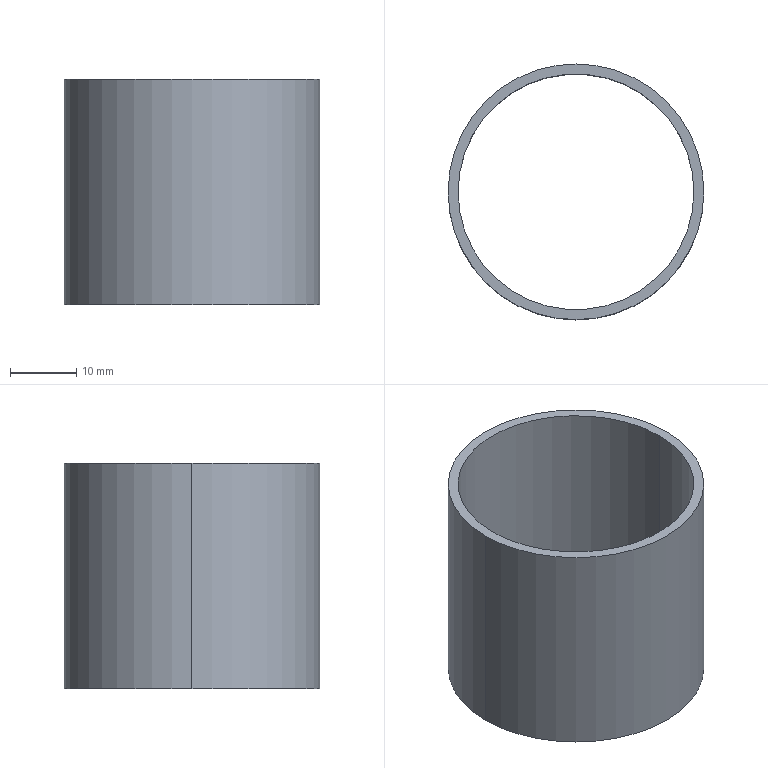Part | STEP file | 20318 | 1 solid | 6 faces | box 38.5 x 38.5 x 34 mm | volume 5928 mm3 | cylinder 4 | plane 2 | commonest cylinder face diameters 35.5 x2 38.5 x2
STEP:
#1=CARTESIAN_POINT('',(19.25,0.,0.));
#2=VERTEX_POINT('',#1);
#3=CARTESIAN_POINT('',(19.25,0.,34.));
#4=VERTEX_POINT('',#3);
#5=CARTESIAN_POINT('',(19.25,0.,17.));
#6=DIRECTION('',(0.,0.,1.));
#7=VECTOR('',#6,1.);
#8=LINE('',#5,#7);
#9=EDGE_CURVE('',#2,#4,#8,.T.);
#10=ORIENTED_EDGE('',*,*,#9,.F.);
#11=CARTESIAN_POINT('',(-19.25,0.,0.));
#12=VERTEX_POINT('',#11);
#13=CARTESIAN_POINT('',(0.,0.,0.));
#14=DIRECTION('',(0.,0.,1.));
#15=AXIS2_PLACEMENT_3D('',#13,#14,$);
#16=CIRCLE('',#15,19.25);
#17=EDGE_CURVE('',#2,#12,#16,.T.);
#18=ORIENTED_EDGE('',*,*,#17,.T.);
#19=CARTESIAN_POINT('',(-19.25,0.,34.));
#20=VERTEX_POINT('',#19);
#21=CARTESIAN_POINT('',(-19.25,0.,17.));
#22=DIRECTION('',(0.,0.,1.));
#23=VECTOR('',#22,1.);
#24=LINE('',#21,#23);
#25=EDGE_CURVE('',#12,#20,#24,.T.);
#26=ORIENTED_EDGE('',*,*,#25,.T.);
#27=CARTESIAN_POINT('',(0.,0.,34.));
#28=DIRECTION('',(0.,0.,1.));
#29=AXIS2_PLACEMENT_3D('',#27,#28,$);
#30=CIRCLE('',#29,19.25);
#31=EDGE_CURVE('',#4,#20,#30,.T.);
#32=ORIENTED_EDGE('',*,*,#31,.F.);
#33=EDGE_LOOP('',(#10,#18,#26,#32));
#34=FACE_OUTER_BOUND('',#33,.T.);
#35=CARTESIAN_POINT('',(0.,0.,17.));
#36=DIRECTION('',(0.,0.,1.));
#37=DIRECTION('',(1.,0.,0.));
#38=AXIS2_PLACEMENT_3D('',#35,#36,#37);
#39=CYLINDRICAL_SURFACE('',#38,19.25);
#40=ADVANCED_FACE('',(#34),#39,.T.);
#41=ORIENTED_EDGE('',*,*,#25,.F.);
#42=CARTESIAN_POINT('',(0.,0.,0.));
#43=DIRECTION('',(0.,0.,1.));
#44=AXIS2_PLACEMENT_3D('',#42,#43,$);
#45=CIRCLE('',#44,19.25);
#46=EDGE_CURVE('',#12,#2,#45,.T.);
#47=ORIENTED_EDGE('',*,*,#46,.T.);
#48=ORIENTED_EDGE('',*,*,#9,.T.);
#49=CARTESIAN_POINT('',(0.,0.,34.));
#50=DIRECTION('',(0.,0.,1.));
#51=AXIS2_PLACEMENT_3D('',#49,#50,$);
#52=CIRCLE('',#51,19.25);
#53=EDGE_CURVE('',#20,#4,#52,.T.);
#54=ORIENTED_EDGE('',*,*,#53,.F.);
#55=EDGE_LOOP('',(#41,#47,#48,#54));
#56=FACE_OUTER_BOUND('',#55,.T.);
#57=ADVANCED_FACE('',(#56),#39,.T.);
#58=CARTESIAN_POINT('',(-17.75,0.,34.));
#59=VERTEX_POINT('',#58);
#60=CARTESIAN_POINT('',(17.75,0.,34.));
#61=VERTEX_POINT('',#60);
#62=CARTESIAN_POINT('',(0.,0.,34.));
#63=DIRECTION('',(0.,0.,1.));
#64=AXIS2_PLACEMENT_3D('',#62,#63,$);
#65=CIRCLE('',#64,17.75);
#66=EDGE_CURVE('',#59,#61,#65,.T.);
#67=ORIENTED_EDGE('',*,*,#66,.T.);
#68=CARTESIAN_POINT('',(17.75,0.,0.));
#69=VERTEX_POINT('',#68);
#70=CARTESIAN_POINT('',(17.75,0.,17.));
#71=DIRECTION('',(0.,0.,1.));
#72=VECTOR('',#71,1.);
#73=LINE('',#70,#72);
#74=EDGE_CURVE('',#69,#61,#73,.T.);
#75=ORIENTED_EDGE('',*,*,#74,.F.);
#76=CARTESIAN_POINT('',(-17.75,0.,0.));
#77=VERTEX_POINT('',#76);
#78=CARTESIAN_POINT('',(0.,0.,0.));
#79=DIRECTION('',(0.,0.,1.));
#80=AXIS2_PLACEMENT_3D('',#78,#79,$);
#81=CIRCLE('',#80,17.75);
#82=EDGE_CURVE('',#77,#69,#81,.T.);
#83=ORIENTED_EDGE('',*,*,#82,.F.);
#84=CARTESIAN_POINT('',(-17.75,0.,17.));
#85=DIRECTION('',(0.,0.,1.));
#86=VECTOR('',#85,1.);
#87=LINE('',#84,#86);
#88=EDGE_CURVE('',#77,#59,#87,.T.);
#89=ORIENTED_EDGE('',*,*,#88,.T.);
#90=EDGE_LOOP('',(#67,#75,#83,#89));
#91=FACE_OUTER_BOUND('',#90,.T.);
#92=CARTESIAN_POINT('',(0.,0.,17.));
#93=DIRECTION('',(0.,0.,1.));
#94=DIRECTION('',(1.,0.,0.));
#95=AXIS2_PLACEMENT_3D('',#92,#93,#94);
#96=CYLINDRICAL_SURFACE('',#95,17.75);
#97=ADVANCED_FACE('',(#91),#96,.F.);
#98=CARTESIAN_POINT('',(0.,0.,34.));
#99=DIRECTION('',(0.,0.,1.));
#100=AXIS2_PLACEMENT_3D('',#98,#99,$);
#101=CIRCLE('',#100,17.75);
#102=EDGE_CURVE('',#61,#59,#101,.T.);
#103=ORIENTED_EDGE('',*,*,#102,.T.);
#104=ORIENTED_EDGE('',*,*,#88,.F.);
#105=CARTESIAN_POINT('',(0.,0.,0.));
#106=DIRECTION('',(0.,0.,1.));
#107=AXIS2_PLACEMENT_3D('',#105,#106,$);
#108=CIRCLE('',#107,17.75);
#109=EDGE_CURVE('',#69,#77,#108,.T.);
#110=ORIENTED_EDGE('',*,*,#109,.F.);
#111=ORIENTED_EDGE('',*,*,#74,.T.);
#112=EDGE_LOOP('',(#103,#104,#110,#111));
#113=FACE_OUTER_BOUND('',#112,.T.);
#114=ADVANCED_FACE('',(#113),#96,.F.);
#115=ORIENTED_EDGE('',*,*,#46,.F.);
#116=ORIENTED_EDGE('',*,*,#17,.F.);
#117=EDGE_LOOP('',(#115,#116));
#118=FACE_OUTER_BOUND('',#117,.T.);
#119=ORIENTED_EDGE('',*,*,#109,.T.);
#120=ORIENTED_EDGE('',*,*,#82,.T.);
#121=EDGE_LOOP('',(#119,#120));
#122=FACE_BOUND('',#121,.T.);
#123=CARTESIAN_POINT('',(0.,0.,0.));
#124=DIRECTION('',(0.,0.,1.));
#125=DIRECTION('',(1.,0.,0.));
#126=AXIS2_PLACEMENT_3D('',#123,#124,#125);
#127=PLANE('',#126);
#128=ADVANCED_FACE('',(#118,#122),#127,.F.);
#129=ORIENTED_EDGE('',*,*,#31,.T.);
#130=ORIENTED_EDGE('',*,*,#53,.T.);
#131=EDGE_LOOP('',(#129,#130));
#132=FACE_OUTER_BOUND('',#131,.T.);
#133=ORIENTED_EDGE('',*,*,#66,.F.);
#134=ORIENTED_EDGE('',*,*,#102,.F.);
#135=EDGE_LOOP('',(#133,#134));
#136=FACE_BOUND('',#135,.T.);
#137=CARTESIAN_POINT('',(0.,0.,34.));
#138=DIRECTION('',(0.,0.,1.));
#139=DIRECTION('',(1.,0.,0.));
#140=AXIS2_PLACEMENT_3D('',#137,#138,#139);
#141=PLANE('',#140);
#142=ADVANCED_FACE('',(#132,#136),#141,.T.);
#143=CLOSED_SHELL('',(#40,#57,#97,#114,#128,#142));
#144=MANIFOLD_SOLID_BREP('',#143);
#145=(LENGTH_UNIT()NAMED_UNIT(*)SI_UNIT(.MILLI.,.METRE.));
#146=UNCERTAINTY_MEASURE_WITH_UNIT(LENGTH_MEASURE(0.005),#145,'','');
#147=(NAMED_UNIT(*)PLANE_ANGLE_UNIT()SI_UNIT($,.RADIAN.));
#148=(NAMED_UNIT(*)SI_UNIT($,.STERADIAN.)SOLID_ANGLE_UNIT());
#149=(GEOMETRIC_REPRESENTATION_CONTEXT(3)GLOBAL_UNCERTAINTY_ASSIGNED_CONTEXT((#146))GLOBAL_UNIT_ASSIGNED_CONTEXT((#145,#147,#148))REPRESENTATION_CONTEXT('',''));
#150=ADVANCED_BREP_SHAPE_REPRESENTATION('',(#144),#149);